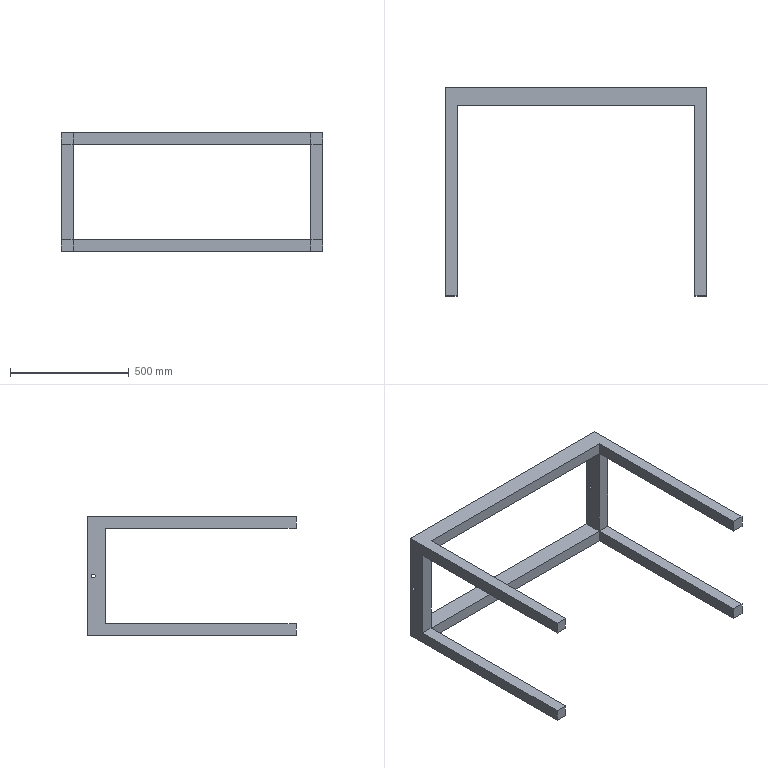Part | SolidWorks | features Cut 1, Extrusion 1, ICE 1 | 1 solid | 29 faces | box 1100 x 875 x 500 mm | volume 19232329 mm3 | plane 25 | cylinder 4 | commonest cylinder face diameters 15 x4
STEP:
#1=CARTESIAN_POINT('',(550.,52.5,-7.5));
#2=VERTEX_POINT('',#1);
#3=CARTESIAN_POINT('',(550.,52.5,7.5));
#4=VERTEX_POINT('',#3);
#5=CARTESIAN_POINT('',(550.,52.5,0.));
#6=DIRECTION('',(-1.,0.,0.));
#7=DIRECTION('',(0.,0.,1.));
#8=AXIS2_PLACEMENT_3D('',#5,#6,#7);
#9=CIRCLE('',#8,7.5);
#10=EDGE_CURVE('',#2,#4,#9,.T.);
#11=ORIENTED_EDGE('',*,*,#10,.F.);
#12=CARTESIAN_POINT('',(500.,52.5,-7.5));
#13=VERTEX_POINT('',#12);
#14=CARTESIAN_POINT('',(550.,52.5,-7.5));
#15=DIRECTION('',(-1.,0.,0.));
#16=VECTOR('',#15,1000.);
#17=LINE('',#14,#16);
#18=EDGE_CURVE('',#2,#13,#17,.T.);
#19=ORIENTED_EDGE('',*,*,#18,.T.);
#20=CARTESIAN_POINT('',(500.,52.5,7.5));
#21=VERTEX_POINT('',#20);
#22=CARTESIAN_POINT('',(500.,52.5,0.));
#23=DIRECTION('',(-1.,0.,0.));
#24=DIRECTION('',(0.,0.,1.));
#25=AXIS2_PLACEMENT_3D('',#22,#23,#24);
#26=CIRCLE('',#25,7.5);
#27=EDGE_CURVE('',#13,#21,#26,.T.);
#28=ORIENTED_EDGE('',*,*,#27,.T.);
#29=CARTESIAN_POINT('',(550.,52.5,7.5));
#30=DIRECTION('',(-1.,0.,0.));
#31=VECTOR('',#30,1000.);
#32=LINE('',#29,#31);
#33=EDGE_CURVE('',#4,#21,#32,.T.);
#34=ORIENTED_EDGE('',*,*,#33,.F.);
#35=EDGE_LOOP('',(#11,#19,#28,#34));
#36=FACE_OUTER_BOUND('',#35,.T.);
#37=CARTESIAN_POINT('',(550.,52.5,0.));
#38=DIRECTION('',(-1.,0.,0.));
#39=DIRECTION('',(0.,0.,1.));
#40=AXIS2_PLACEMENT_3D('',#37,#38,#39);
#41=CYLINDRICAL_SURFACE('',#40,7.5);
#42=ADVANCED_FACE('',(#36),#41,.F.);
#43=CARTESIAN_POINT('',(-500.,52.5,7.5));
#44=VERTEX_POINT('',#43);
#45=CARTESIAN_POINT('',(-500.,52.5,-7.5));
#46=VERTEX_POINT('',#45);
#47=CARTESIAN_POINT('',(-500.,52.5,0.));
#48=DIRECTION('',(1.,0.,0.));
#49=DIRECTION('',(0.,0.,-1.));
#50=AXIS2_PLACEMENT_3D('',#47,#48,#49);
#51=CIRCLE('',#50,7.5);
#52=EDGE_CURVE('',#44,#46,#51,.T.);
#53=ORIENTED_EDGE('',*,*,#52,.T.);
#54=CARTESIAN_POINT('',(-550.,52.5,-7.5));
#55=VERTEX_POINT('',#54);
#56=CARTESIAN_POINT('',(550.,52.5,-7.5));
#57=DIRECTION('',(-1.,0.,0.));
#58=VECTOR('',#57,1000.);
#59=LINE('',#56,#58);
#60=EDGE_CURVE('',#46,#55,#59,.T.);
#61=ORIENTED_EDGE('',*,*,#60,.T.);
#62=CARTESIAN_POINT('',(-550.,52.5,7.5));
#63=VERTEX_POINT('',#62);
#64=CARTESIAN_POINT('',(-550.,52.5,0.));
#65=DIRECTION('',(1.,0.,0.));
#66=DIRECTION('',(0.,0.,-1.));
#67=AXIS2_PLACEMENT_3D('',#64,#65,#66);
#68=CIRCLE('',#67,7.5);
#69=EDGE_CURVE('',#63,#55,#68,.T.);
#70=ORIENTED_EDGE('',*,*,#69,.F.);
#71=CARTESIAN_POINT('',(550.,52.5,7.5));
#72=DIRECTION('',(-1.,0.,0.));
#73=VECTOR('',#72,1000.);
#74=LINE('',#71,#73);
#75=EDGE_CURVE('',#44,#63,#74,.T.);
#76=ORIENTED_EDGE('',*,*,#75,.F.);
#77=EDGE_LOOP('',(#53,#61,#70,#76));
#78=FACE_OUTER_BOUND('',#77,.T.);
#79=CARTESIAN_POINT('',(550.,52.5,0.));
#80=DIRECTION('',(-1.,0.,0.));
#81=DIRECTION('',(0.,0.,1.));
#82=AXIS2_PLACEMENT_3D('',#79,#80,#81);
#83=CYLINDRICAL_SURFACE('',#82,7.5);
#84=ADVANCED_FACE('',(#78),#83,.F.);
#85=CARTESIAN_POINT('',(-500.,0.,-200.));
#86=VERTEX_POINT('',#85);
#87=CARTESIAN_POINT('',(-550.,0.,-200.));
#88=VERTEX_POINT('',#87);
#89=CARTESIAN_POINT('',(-550.,0.,-200.));
#90=DIRECTION('',(-1.,0.,0.));
#91=VECTOR('',#90,1000.);
#92=LINE('',#89,#91);
#93=EDGE_CURVE('',#86,#88,#92,.T.);
#94=ORIENTED_EDGE('',*,*,#93,.F.);
#95=CARTESIAN_POINT('',(-500.,0.,200.));
#96=VERTEX_POINT('',#95);
#97=CARTESIAN_POINT('',(-500.,0.,200.));
#98=DIRECTION('',(0.,0.,1.));
#99=VECTOR('',#98,1000.);
#100=LINE('',#97,#99);
#101=EDGE_CURVE('',#86,#96,#100,.T.);
#102=ORIENTED_EDGE('',*,*,#101,.T.);
#103=CARTESIAN_POINT('',(-550.,0.,200.));
#104=VERTEX_POINT('',#103);
#105=CARTESIAN_POINT('',(-550.,0.,200.));
#106=DIRECTION('',(1.,0.,0.));
#107=VECTOR('',#106,1000.);
#108=LINE('',#105,#107);
#109=EDGE_CURVE('',#104,#96,#108,.T.);
#110=ORIENTED_EDGE('',*,*,#109,.F.);
#111=CARTESIAN_POINT('',(-550.,0.,250.));
#112=DIRECTION('',(0.,0.,1.));
#113=VECTOR('',#112,1000.);
#114=LINE('',#111,#113);
#115=EDGE_CURVE('',#88,#104,#114,.T.);
#116=ORIENTED_EDGE('',*,*,#115,.F.);
#117=EDGE_LOOP('',(#94,#102,#110,#116));
#118=FACE_OUTER_BOUND('',#117,.T.);
#119=CARTESIAN_POINT('',(0.,0.,0.));
#120=DIRECTION('',(0.,-1.,0.));
#121=DIRECTION('',(0.,0.,-1.));
#122=AXIS2_PLACEMENT_3D('',#119,#120,#121);
#123=PLANE('',#122);
#124=ADVANCED_FACE('',(#118),#123,.T.);
#125=CARTESIAN_POINT('',(500.,0.,200.));
#126=VERTEX_POINT('',#125);
#127=CARTESIAN_POINT('',(550.,0.,200.));
#128=VERTEX_POINT('',#127);
#129=CARTESIAN_POINT('',(550.,0.,200.));
#130=DIRECTION('',(1.,0.,0.));
#131=VECTOR('',#130,1000.);
#132=LINE('',#129,#131);
#133=EDGE_CURVE('',#126,#128,#132,.T.);
#134=ORIENTED_EDGE('',*,*,#133,.F.);
#135=CARTESIAN_POINT('',(500.,0.,-200.));
#136=VERTEX_POINT('',#135);
#137=CARTESIAN_POINT('',(500.,0.,200.));
#138=DIRECTION('',(0.,0.,-1.));
#139=VECTOR('',#138,1000.);
#140=LINE('',#137,#139);
#141=EDGE_CURVE('',#126,#136,#140,.T.);
#142=ORIENTED_EDGE('',*,*,#141,.T.);
#143=CARTESIAN_POINT('',(550.,0.,-200.));
#144=VERTEX_POINT('',#143);
#145=CARTESIAN_POINT('',(550.,0.,-200.));
#146=DIRECTION('',(-1.,0.,0.));
#147=VECTOR('',#146,1000.);
#148=LINE('',#145,#147);
#149=EDGE_CURVE('',#144,#136,#148,.T.);
#150=ORIENTED_EDGE('',*,*,#149,.F.);
#151=CARTESIAN_POINT('',(550.,0.,250.));
#152=DIRECTION('',(0.,0.,-1.));
#153=VECTOR('',#152,1000.);
#154=LINE('',#151,#153);
#155=EDGE_CURVE('',#128,#144,#154,.T.);
#156=ORIENTED_EDGE('',*,*,#155,.F.);
#157=EDGE_LOOP('',(#134,#142,#150,#156));
#158=FACE_OUTER_BOUND('',#157,.T.);
#159=CARTESIAN_POINT('',(0.,0.,0.));
#160=DIRECTION('',(0.,-1.,0.));
#161=DIRECTION('',(0.,0.,-1.));
#162=AXIS2_PLACEMENT_3D('',#159,#160,#161);
#163=PLANE('',#162);
#164=ADVANCED_FACE('',(#158),#163,.T.);
#165=CARTESIAN_POINT('',(-500.,0.,-250.));
#166=VERTEX_POINT('',#165);
#167=CARTESIAN_POINT('',(-500.,0.,-250.));
#168=DIRECTION('',(0.,0.,1.));
#169=VECTOR('',#168,1000.);
#170=LINE('',#167,#169);
#171=EDGE_CURVE('',#166,#86,#170,.T.);
#172=ORIENTED_EDGE('',*,*,#171,.F.);
#173=CARTESIAN_POINT('',(500.,0.,-250.));
#174=VERTEX_POINT('',#173);
#175=CARTESIAN_POINT('',(-550.,0.,-250.));
#176=DIRECTION('',(-1.,0.,0.));
#177=VECTOR('',#176,1000.);
#178=LINE('',#175,#177);
#179=EDGE_CURVE('',#174,#166,#178,.T.);
#180=ORIENTED_EDGE('',*,*,#179,.F.);
#181=CARTESIAN_POINT('',(500.,0.,-250.));
#182=DIRECTION('',(0.,0.,-1.));
#183=VECTOR('',#182,1000.);
#184=LINE('',#181,#183);
#185=EDGE_CURVE('',#136,#174,#184,.T.);
#186=ORIENTED_EDGE('',*,*,#185,.F.);
#187=CARTESIAN_POINT('',(-500.,0.,-200.));
#188=DIRECTION('',(-1.,0.,0.));
#189=VECTOR('',#188,1000.);
#190=LINE('',#187,#189);
#191=EDGE_CURVE('',#136,#86,#190,.T.);
#192=ORIENTED_EDGE('',*,*,#191,.T.);
#193=EDGE_LOOP('',(#172,#180,#186,#192));
#194=FACE_OUTER_BOUND('',#193,.T.);
#195=CARTESIAN_POINT('',(0.,0.,0.));
#196=DIRECTION('',(0.,-1.,0.));
#197=DIRECTION('',(0.,0.,-1.));
#198=AXIS2_PLACEMENT_3D('',#195,#196,#197);
#199=PLANE('',#198);
#200=ADVANCED_FACE('',(#194),#199,.T.);
#201=CARTESIAN_POINT('',(550.,75.,250.));
#202=VERTEX_POINT('',#201);
#203=CARTESIAN_POINT('',(550.,75.,-250.));
#204=VERTEX_POINT('',#203);
#205=CARTESIAN_POINT('',(550.,75.,250.));
#206=DIRECTION('',(0.,0.,-1.));
#207=VECTOR('',#206,1000.);
#208=LINE('',#205,#207);
#209=EDGE_CURVE('',#202,#204,#208,.T.);
#210=ORIENTED_EDGE('',*,*,#209,.T.);
#211=CARTESIAN_POINT('',(-550.,75.,-250.));
#212=VERTEX_POINT('',#211);
#213=CARTESIAN_POINT('',(-550.,75.,-250.));
#214=DIRECTION('',(-1.,0.,0.));
#215=VECTOR('',#214,1000.);
#216=LINE('',#213,#215);
#217=EDGE_CURVE('',#204,#212,#216,.T.);
#218=ORIENTED_EDGE('',*,*,#217,.T.);
#219=CARTESIAN_POINT('',(-550.,75.,250.));
#220=VERTEX_POINT('',#219);
#221=CARTESIAN_POINT('',(-550.,75.,250.));
#222=DIRECTION('',(0.,0.,1.));
#223=VECTOR('',#222,1000.);
#224=LINE('',#221,#223);
#225=EDGE_CURVE('',#212,#220,#224,.T.);
#226=ORIENTED_EDGE('',*,*,#225,.T.);
#227=CARTESIAN_POINT('',(-550.,75.,250.));
#228=DIRECTION('',(1.,0.,0.));
#229=VECTOR('',#228,1000.);
#230=LINE('',#227,#229);
#231=EDGE_CURVE('',#220,#202,#230,.T.);
#232=ORIENTED_EDGE('',*,*,#231,.T.);
#233=EDGE_LOOP('',(#210,#218,#226,#232));
#234=FACE_OUTER_BOUND('',#233,.T.);
#235=CARTESIAN_POINT('',(500.,75.,200.));
#236=VERTEX_POINT('',#235);
#237=CARTESIAN_POINT('',(500.,75.,-200.));
#238=VERTEX_POINT('',#237);
#239=CARTESIAN_POINT('',(500.,75.,200.));
#240=DIRECTION('',(0.,0.,-1.));
#241=VECTOR('',#240,1000.);
#242=LINE('',#239,#241);
#243=EDGE_CURVE('',#236,#238,#242,.T.);
#244=ORIENTED_EDGE('',*,*,#243,.F.);
#245=CARTESIAN_POINT('',(-500.,75.,200.));
#246=VERTEX_POINT('',#245);
#247=CARTESIAN_POINT('',(-500.,75.,200.));
#248=DIRECTION('',(1.,0.,0.));
#249=VECTOR('',#248,1000.);
#250=LINE('',#247,#249);
#251=EDGE_CURVE('',#246,#236,#250,.T.);
#252=ORIENTED_EDGE('',*,*,#251,.F.);
#253=CARTESIAN_POINT('',(-500.,75.,-200.));
#254=VERTEX_POINT('',#253);
#255=CARTESIAN_POINT('',(-500.,75.,200.));
#256=DIRECTION('',(0.,0.,1.));
#257=VECTOR('',#256,1000.);
#258=LINE('',#255,#257);
#259=EDGE_CURVE('',#254,#246,#258,.T.);
#260=ORIENTED_EDGE('',*,*,#259,.F.);
#261=CARTESIAN_POINT('',(-500.,75.,-200.));
#262=DIRECTION('',(-1.,0.,0.));
#263=VECTOR('',#262,1000.);
#264=LINE('',#261,#263);
#265=EDGE_CURVE('',#238,#254,#264,.T.);
#266=ORIENTED_EDGE('',*,*,#265,.F.);
#267=EDGE_LOOP('',(#244,#252,#260,#266));
#268=FACE_BOUND('',#267,.T.);
#269=CARTESIAN_POINT('',(0.,75.,0.));
#270=DIRECTION('',(0.,-1.,0.));
#271=DIRECTION('',(0.,0.,-1.));
#272=AXIS2_PLACEMENT_3D('',#269,#270,#271);
#273=PLANE('',#272);
#274=ADVANCED_FACE('',(#234,#268),#273,.F.);
#275=CARTESIAN_POINT('',(500.,0.,250.));
#276=VERTEX_POINT('',#275);
#277=CARTESIAN_POINT('',(500.,0.,250.));
#278=DIRECTION('',(0.,0.,-1.));
#279=VECTOR('',#278,1000.);
#280=LINE('',#277,#279);
#281=EDGE_CURVE('',#276,#126,#280,.T.);
#282=ORIENTED_EDGE('',*,*,#281,.F.);
#283=CARTESIAN_POINT('',(-500.,0.,250.));
#284=VERTEX_POINT('',#283);
#285=CARTESIAN_POINT('',(-550.,0.,250.));
#286=DIRECTION('',(1.,0.,0.));
#287=VECTOR('',#286,1000.);
#288=LINE('',#285,#287);
#289=EDGE_CURVE('',#284,#276,#288,.T.);
#290=ORIENTED_EDGE('',*,*,#289,.F.);
#291=CARTESIAN_POINT('',(-500.,0.,250.));
#292=DIRECTION('',(0.,0.,1.));
#293=VECTOR('',#292,1000.);
#294=LINE('',#291,#293);
#295=EDGE_CURVE('',#96,#284,#294,.T.);
#296=ORIENTED_EDGE('',*,*,#295,.F.);
#297=CARTESIAN_POINT('',(-500.,0.,200.));
#298=DIRECTION('',(1.,0.,0.));
#299=VECTOR('',#298,1000.);
#300=LINE('',#297,#299);
#301=EDGE_CURVE('',#96,#126,#300,.T.);
#302=ORIENTED_EDGE('',*,*,#301,.T.);
#303=EDGE_LOOP('',(#282,#290,#296,#302));
#304=FACE_OUTER_BOUND('',#303,.T.);
#305=CARTESIAN_POINT('',(0.,0.,0.));
#306=DIRECTION('',(0.,-1.,0.));
#307=DIRECTION('',(0.,0.,-1.));
#308=AXIS2_PLACEMENT_3D('',#305,#306,#307);
#309=PLANE('',#308);
#310=ADVANCED_FACE('',(#304),#309,.T.);
#311=CARTESIAN_POINT('',(550.,52.5,0.));
#312=DIRECTION('',(-1.,0.,0.));
#313=DIRECTION('',(0.,0.,1.));
#314=AXIS2_PLACEMENT_3D('',#311,#312,#313);
#315=CIRCLE('',#314,7.5);
#316=EDGE_CURVE('',#4,#2,#315,.T.);
#317=ORIENTED_EDGE('',*,*,#316,.T.);
#318=ORIENTED_EDGE('',*,*,#10,.T.);
#319=EDGE_LOOP('',(#317,#318));
#320=FACE_BOUND('',#319,.T.);
#321=CARTESIAN_POINT('',(550.,-800.,250.));
#322=VERTEX_POINT('',#321);
#323=CARTESIAN_POINT('',(550.,75.,250.));
#324=DIRECTION('',(0.,-1.,0.));
#325=VECTOR('',#324,1000.);
#326=LINE('',#323,#325);
#327=EDGE_CURVE('',#202,#322,#326,.T.);
#328=ORIENTED_EDGE('',*,*,#327,.T.);
#329=CARTESIAN_POINT('',(550.,-800.,200.));
#330=VERTEX_POINT('',#329);
#331=CARTESIAN_POINT('',(550.,-800.,250.));
#332=DIRECTION('',(0.,0.,1.));
#333=VECTOR('',#332,1000.);
#334=LINE('',#331,#333);
#335=EDGE_CURVE('',#330,#322,#334,.T.);
#336=ORIENTED_EDGE('',*,*,#335,.F.);
#337=CARTESIAN_POINT('',(550.,-800.,200.));
#338=DIRECTION('',(0.,1.,0.));
#339=VECTOR('',#338,1000.);
#340=LINE('',#337,#339);
#341=EDGE_CURVE('',#330,#128,#340,.T.);
#342=ORIENTED_EDGE('',*,*,#341,.T.);
#343=ORIENTED_EDGE('',*,*,#155,.T.);
#344=CARTESIAN_POINT('',(550.,-800.,-200.));
#345=VERTEX_POINT('',#344);
#346=CARTESIAN_POINT('',(550.,-800.,-200.));
#347=DIRECTION('',(0.,1.,0.));
#348=VECTOR('',#347,1000.);
#349=LINE('',#346,#348);
#350=EDGE_CURVE('',#345,#144,#349,.T.);
#351=ORIENTED_EDGE('',*,*,#350,.F.);
#352=CARTESIAN_POINT('',(550.,-800.,-250.));
#353=VERTEX_POINT('',#352);
#354=CARTESIAN_POINT('',(550.,-800.,-250.));
#355=DIRECTION('',(0.,0.,1.));
#356=VECTOR('',#355,1000.);
#357=LINE('',#354,#356);
#358=EDGE_CURVE('',#353,#345,#357,.T.);
#359=ORIENTED_EDGE('',*,*,#358,.F.);
#360=CARTESIAN_POINT('',(550.,75.,-250.));
#361=DIRECTION('',(0.,-1.,0.));
#362=VECTOR('',#361,1000.);
#363=LINE('',#360,#362);
#364=EDGE_CURVE('',#204,#353,#363,.T.);
#365=ORIENTED_EDGE('',*,*,#364,.F.);
#366=ORIENTED_EDGE('',*,*,#209,.F.);
#367=EDGE_LOOP('',(#328,#336,#342,#343,#351,#359,#365,#366));
#368=FACE_OUTER_BOUND('',#367,.T.);
#369=CARTESIAN_POINT('',(550.,75.,250.));
#370=DIRECTION('',(-1.,0.,0.));
#371=DIRECTION('',(0.,0.,1.));
#372=AXIS2_PLACEMENT_3D('',#369,#370,#371);
#373=PLANE('',#372);
#374=ADVANCED_FACE('',(#320,#368),#373,.F.);
#375=ORIENTED_EDGE('',*,*,#364,.T.);
#376=CARTESIAN_POINT('',(500.,-800.,-250.));
#377=VERTEX_POINT('',#376);
#378=CARTESIAN_POINT('',(550.,-800.,-250.));
#379=DIRECTION('',(1.,0.,0.));
#380=VECTOR('',#379,1000.);
#381=LINE('',#378,#380);
#382=EDGE_CURVE('',#377,#353,#381,.T.);
#383=ORIENTED_EDGE('',*,*,#382,.F.);
#384=CARTESIAN_POINT('',(500.,-800.,-250.));
#385=DIRECTION('',(0.,1.,0.));
#386=VECTOR('',#385,1000.);
#387=LINE('',#384,#386);
#388=EDGE_CURVE('',#377,#174,#387,.T.);
#389=ORIENTED_EDGE('',*,*,#388,.T.);
#390=ORIENTED_EDGE('',*,*,#179,.T.);
#391=CARTESIAN_POINT('',(-500.,-800.,-250.));
#392=VERTEX_POINT('',#391);
#393=CARTESIAN_POINT('',(-500.,-800.,-250.));
#394=DIRECTION('',(0.,1.,0.));
#395=VECTOR('',#394,1000.);
#396=LINE('',#393,#395);
#397=EDGE_CURVE('',#392,#166,#396,.T.);
#398=ORIENTED_EDGE('',*,*,#397,.F.);
#399=CARTESIAN_POINT('',(-550.,-800.,-250.));
#400=VERTEX_POINT('',#399);
#401=CARTESIAN_POINT('',(-550.,-800.,-250.));
#402=DIRECTION('',(1.,0.,0.));
#403=VECTOR('',#402,1000.);
#404=LINE('',#401,#403);
#405=EDGE_CURVE('',#400,#392,#404,.T.);
#406=ORIENTED_EDGE('',*,*,#405,.F.);
#407=CARTESIAN_POINT('',(-550.,75.,-250.));
#408=DIRECTION('',(0.,-1.,0.));
#409=VECTOR('',#408,1000.);
#410=LINE('',#407,#409);
#411=EDGE_CURVE('',#212,#400,#410,.T.);
#412=ORIENTED_EDGE('',*,*,#411,.F.);
#413=ORIENTED_EDGE('',*,*,#217,.F.);
#414=EDGE_LOOP('',(#375,#383,#389,#390,#398,#406,#412,#413));
#415=FACE_OUTER_BOUND('',#414,.T.);
#416=CARTESIAN_POINT('',(-550.,75.,-250.));
#417=DIRECTION('',(0.,0.,1.));
#418=DIRECTION('',(1.,0.,0.));
#419=AXIS2_PLACEMENT_3D('',#416,#417,#418);
#420=PLANE('',#419);
#421=ADVANCED_FACE('',(#415),#420,.F.);
#422=ORIENTED_EDGE('',*,*,#69,.T.);
#423=CARTESIAN_POINT('',(-550.,52.5,0.));
#424=DIRECTION('',(1.,0.,0.));
#425=DIRECTION('',(0.,0.,-1.));
#426=AXIS2_PLACEMENT_3D('',#423,#424,#425);
#427=CIRCLE('',#426,7.5);
#428=EDGE_CURVE('',#55,#63,#427,.T.);
#429=ORIENTED_EDGE('',*,*,#428,.T.);
#430=EDGE_LOOP('',(#422,#429));
#431=FACE_BOUND('',#430,.T.);
#432=ORIENTED_EDGE('',*,*,#411,.T.);
#433=CARTESIAN_POINT('',(-550.,-800.,-200.));
#434=VERTEX_POINT('',#433);
#435=CARTESIAN_POINT('',(-550.,-800.,-250.));
#436=DIRECTION('',(0.,0.,-1.));
#437=VECTOR('',#436,1000.);
#438=LINE('',#435,#437);
#439=EDGE_CURVE('',#434,#400,#438,.T.);
#440=ORIENTED_EDGE('',*,*,#439,.F.);
#441=CARTESIAN_POINT('',(-550.,-800.,-200.));
#442=DIRECTION('',(0.,1.,0.));
#443=VECTOR('',#442,1000.);
#444=LINE('',#441,#443);
#445=EDGE_CURVE('',#434,#88,#444,.T.);
#446=ORIENTED_EDGE('',*,*,#445,.T.);
#447=ORIENTED_EDGE('',*,*,#115,.T.);
#448=CARTESIAN_POINT('',(-550.,-800.,200.));
#449=VERTEX_POINT('',#448);
#450=CARTESIAN_POINT('',(-550.,-800.,200.));
#451=DIRECTION('',(0.,1.,0.));
#452=VECTOR('',#451,1000.);
#453=LINE('',#450,#452);
#454=EDGE_CURVE('',#449,#104,#453,.T.);
#455=ORIENTED_EDGE('',*,*,#454,.F.);
#456=CARTESIAN_POINT('',(-550.,-800.,250.));
#457=VERTEX_POINT('',#456);
#458=CARTESIAN_POINT('',(-550.,-800.,250.));
#459=DIRECTION('',(0.,0.,-1.));
#460=VECTOR('',#459,1000.);
#461=LINE('',#458,#460);
#462=EDGE_CURVE('',#457,#449,#461,.T.);
#463=ORIENTED_EDGE('',*,*,#462,.F.);
#464=CARTESIAN_POINT('',(-550.,75.,250.));
#465=DIRECTION('',(0.,-1.,0.));
#466=VECTOR('',#465,1000.);
#467=LINE('',#464,#466);
#468=EDGE_CURVE('',#220,#457,#467,.T.);
#469=ORIENTED_EDGE('',*,*,#468,.F.);
#470=ORIENTED_EDGE('',*,*,#225,.F.);
#471=EDGE_LOOP('',(#432,#440,#446,#447,#455,#463,#469,#470));
#472=FACE_OUTER_BOUND('',#471,.T.);
#473=CARTESIAN_POINT('',(-550.,75.,250.));
#474=DIRECTION('',(1.,0.,0.));
#475=DIRECTION('',(0.,0.,-1.));
#476=AXIS2_PLACEMENT_3D('',#473,#474,#475);
#477=PLANE('',#476);
#478=ADVANCED_FACE('',(#431,#472),#477,.F.);
#479=ORIENTED_EDGE('',*,*,#468,.T.);
#480=CARTESIAN_POINT('',(-500.,-800.,250.));
#481=VERTEX_POINT('',#480);
#482=CARTESIAN_POINT('',(-550.,-800.,250.));
#483=DIRECTION('',(-1.,0.,0.));
#484=VECTOR('',#483,1000.);
#485=LINE('',#482,#484);
#486=EDGE_CURVE('',#481,#457,#485,.T.);
#487=ORIENTED_EDGE('',*,*,#486,.F.);
#488=CARTESIAN_POINT('',(-500.,-800.,250.));
#489=DIRECTION('',(0.,1.,0.));
#490=VECTOR('',#489,1000.);
#491=LINE('',#488,#490);
#492=EDGE_CURVE('',#481,#284,#491,.T.);
#493=ORIENTED_EDGE('',*,*,#492,.T.);
#494=ORIENTED_EDGE('',*,*,#289,.T.);
#495=CARTESIAN_POINT('',(500.,-800.,250.));
#496=VERTEX_POINT('',#495);
#497=CARTESIAN_POINT('',(500.,-800.,250.));
#498=DIRECTION('',(0.,1.,0.));
#499=VECTOR('',#498,1000.);
#500=LINE('',#497,#499);
#501=EDGE_CURVE('',#496,#276,#500,.T.);
#502=ORIENTED_EDGE('',*,*,#501,.F.);
#503=CARTESIAN_POINT('',(550.,-800.,250.));
#504=DIRECTION('',(-1.,0.,0.));
#505=VECTOR('',#504,1000.);
#506=LINE('',#503,#505);
#507=EDGE_CURVE('',#322,#496,#506,.T.);
#508=ORIENTED_EDGE('',*,*,#507,.F.);
#509=ORIENTED_EDGE('',*,*,#327,.F.);
#510=ORIENTED_EDGE('',*,*,#231,.F.);
#511=EDGE_LOOP('',(#479,#487,#493,#494,#502,#508,#509,#510));
#512=FACE_OUTER_BOUND('',#511,.T.);
#513=CARTESIAN_POINT('',(-550.,75.,250.));
#514=DIRECTION('',(0.,0.,-1.));
#515=DIRECTION('',(-1.,0.,0.));
#516=AXIS2_PLACEMENT_3D('',#513,#514,#515);
#517=PLANE('',#516);
#518=ADVANCED_FACE('',(#512),#517,.F.);
#519=CARTESIAN_POINT('',(500.,52.5,0.));
#520=DIRECTION('',(-1.,0.,0.));
#521=DIRECTION('',(0.,0.,1.));
#522=AXIS2_PLACEMENT_3D('',#519,#520,#521);
#523=CIRCLE('',#522,7.5);
#524=EDGE_CURVE('',#21,#13,#523,.T.);
#525=ORIENTED_EDGE('',*,*,#524,.F.);
#526=ORIENTED_EDGE('',*,*,#27,.F.);
#527=EDGE_LOOP('',(#525,#526));
#528=FACE_BOUND('',#527,.T.);
#529=ORIENTED_EDGE('',*,*,#141,.F.);
#530=CARTESIAN_POINT('',(500.,75.,200.));
#531=DIRECTION('',(0.,-1.,0.));
#532=VECTOR('',#531,1000.);
#533=LINE('',#530,#532);
#534=EDGE_CURVE('',#236,#126,#533,.T.);
#535=ORIENTED_EDGE('',*,*,#534,.F.);
#536=ORIENTED_EDGE('',*,*,#243,.T.);
#537=CARTESIAN_POINT('',(500.,75.,-200.));
#538=DIRECTION('',(0.,-1.,0.));
#539=VECTOR('',#538,1000.);
#540=LINE('',#537,#539);
#541=EDGE_CURVE('',#238,#136,#540,.T.);
#542=ORIENTED_EDGE('',*,*,#541,.T.);
#543=EDGE_LOOP('',(#529,#535,#536,#542));
#544=FACE_OUTER_BOUND('',#543,.T.);
#545=CARTESIAN_POINT('',(500.,75.,200.));
#546=DIRECTION('',(-1.,0.,0.));
#547=DIRECTION('',(0.,0.,1.));
#548=AXIS2_PLACEMENT_3D('',#545,#546,#547);
#549=PLANE('',#548);
#550=ADVANCED_FACE('',(#528,#544),#549,.T.);
#551=ORIENTED_EDGE('',*,*,#191,.F.);
#552=ORIENTED_EDGE('',*,*,#541,.F.);
#553=ORIENTED_EDGE('',*,*,#265,.T.);
#554=CARTESIAN_POINT('',(-500.,75.,-200.));
#555=DIRECTION('',(0.,-1.,0.));
#556=VECTOR('',#555,1000.);
#557=LINE('',#554,#556);
#558=EDGE_CURVE('',#254,#86,#557,.T.);
#559=ORIENTED_EDGE('',*,*,#558,.T.);
#560=EDGE_LOOP('',(#551,#552,#553,#559));
#561=FACE_OUTER_BOUND('',#560,.T.);
#562=CARTESIAN_POINT('',(-500.,75.,-200.));
#563=DIRECTION('',(0.,0.,1.));
#564=DIRECTION('',(1.,0.,0.));
#565=AXIS2_PLACEMENT_3D('',#562,#563,#564);
#566=PLANE('',#565);
#567=ADVANCED_FACE('',(#561),#566,.T.);
#568=ORIENTED_EDGE('',*,*,#52,.F.);
#569=CARTESIAN_POINT('',(-500.,52.5,0.));
#570=DIRECTION('',(1.,0.,0.));
#571=DIRECTION('',(0.,0.,-1.));
#572=AXIS2_PLACEMENT_3D('',#569,#570,#571);
#573=CIRCLE('',#572,7.5);
#574=EDGE_CURVE('',#46,#44,#573,.T.);
#575=ORIENTED_EDGE('',*,*,#574,.F.);
#576=EDGE_LOOP('',(#568,#575));
#577=FACE_BOUND('',#576,.T.);
#578=ORIENTED_EDGE('',*,*,#101,.F.);
#579=ORIENTED_EDGE('',*,*,#558,.F.);
#580=ORIENTED_EDGE('',*,*,#259,.T.);
#581=CARTESIAN_POINT('',(-500.,75.,200.));
#582=DIRECTION('',(0.,-1.,0.));
#583=VECTOR('',#582,1000.);
#584=LINE('',#581,#583);
#585=EDGE_CURVE('',#246,#96,#584,.T.);
#586=ORIENTED_EDGE('',*,*,#585,.T.);
#587=EDGE_LOOP('',(#578,#579,#580,#586));
#588=FACE_OUTER_BOUND('',#587,.T.);
#589=CARTESIAN_POINT('',(-500.,75.,200.));
#590=DIRECTION('',(1.,0.,0.));
#591=DIRECTION('',(0.,0.,-1.));
#592=AXIS2_PLACEMENT_3D('',#589,#590,#591);
#593=PLANE('',#592);
#594=ADVANCED_FACE('',(#577,#588),#593,.T.);
#595=ORIENTED_EDGE('',*,*,#301,.F.);
#596=ORIENTED_EDGE('',*,*,#585,.F.);
#597=ORIENTED_EDGE('',*,*,#251,.T.);
#598=ORIENTED_EDGE('',*,*,#534,.T.);
#599=EDGE_LOOP('',(#595,#596,#597,#598));
#600=FACE_OUTER_BOUND('',#599,.T.);
#601=CARTESIAN_POINT('',(-500.,75.,200.));
#602=DIRECTION('',(0.,0.,-1.));
#603=DIRECTION('',(-1.,0.,0.));
#604=AXIS2_PLACEMENT_3D('',#601,#602,#603);
#605=PLANE('',#604);
#606=ADVANCED_FACE('',(#600),#605,.T.);
#607=ORIENTED_EDGE('',*,*,#109,.T.);
#608=CARTESIAN_POINT('',(-500.,-800.,200.));
#609=VERTEX_POINT('',#608);
#610=CARTESIAN_POINT('',(-500.,-800.,200.));
#611=DIRECTION('',(0.,1.,0.));
#612=VECTOR('',#611,1000.);
#613=LINE('',#610,#612);
#614=EDGE_CURVE('',#609,#96,#613,.T.);
#615=ORIENTED_EDGE('',*,*,#614,.F.);
#616=CARTESIAN_POINT('',(-550.,-800.,200.));
#617=DIRECTION('',(1.,0.,0.));
#618=VECTOR('',#617,1000.);
#619=LINE('',#616,#618);
#620=EDGE_CURVE('',#449,#609,#619,.T.);
#621=ORIENTED_EDGE('',*,*,#620,.F.);
#622=ORIENTED_EDGE('',*,*,#454,.T.);
#623=EDGE_LOOP('',(#607,#615,#621,#622));
#624=FACE_OUTER_BOUND('',#623,.T.);
#625=CARTESIAN_POINT('',(-550.,-800.,200.));
#626=DIRECTION('',(0.,0.,1.));
#627=DIRECTION('',(1.,0.,0.));
#628=AXIS2_PLACEMENT_3D('',#625,#626,#627);
#629=PLANE('',#628);
#630=ADVANCED_FACE('',(#624),#629,.F.);
#631=ORIENTED_EDGE('',*,*,#295,.T.);
#632=ORIENTED_EDGE('',*,*,#492,.F.);
#633=CARTESIAN_POINT('',(-500.,-800.,250.));
#634=DIRECTION('',(0.,0.,1.));
#635=VECTOR('',#634,1000.);
#636=LINE('',#633,#635);
#637=EDGE_CURVE('',#609,#481,#636,.T.);
#638=ORIENTED_EDGE('',*,*,#637,.F.);
#639=ORIENTED_EDGE('',*,*,#614,.T.);
#640=EDGE_LOOP('',(#631,#632,#638,#639));
#641=FACE_OUTER_BOUND('',#640,.T.);
#642=CARTESIAN_POINT('',(-500.,-800.,250.));
#643=DIRECTION('',(-1.,0.,0.));
#644=DIRECTION('',(0.,0.,1.));
#645=AXIS2_PLACEMENT_3D('',#642,#643,#644);
#646=PLANE('',#645);
#647=ADVANCED_FACE('',(#641),#646,.F.);
#648=ORIENTED_EDGE('',*,*,#462,.T.);
#649=ORIENTED_EDGE('',*,*,#620,.T.);
#650=ORIENTED_EDGE('',*,*,#637,.T.);
#651=ORIENTED_EDGE('',*,*,#486,.T.);
#652=EDGE_LOOP('',(#648,#649,#650,#651));
#653=FACE_OUTER_BOUND('',#652,.T.);
#654=CARTESIAN_POINT('',(0.,-800.,0.));
#655=DIRECTION('',(0.,-1.,0.));
#656=DIRECTION('',(0.,0.,-1.));
#657=AXIS2_PLACEMENT_3D('',#654,#655,#656);
#658=PLANE('',#657);
#659=ADVANCED_FACE('',(#653),#658,.T.);
#660=ORIENTED_EDGE('',*,*,#149,.T.);
#661=CARTESIAN_POINT('',(500.,-800.,-200.));
#662=VERTEX_POINT('',#661);
#663=CARTESIAN_POINT('',(500.,-800.,-200.));
#664=DIRECTION('',(0.,1.,0.));
#665=VECTOR('',#664,1000.);
#666=LINE('',#663,#665);
#667=EDGE_CURVE('',#662,#136,#666,.T.);
#668=ORIENTED_EDGE('',*,*,#667,.F.);
#669=CARTESIAN_POINT('',(550.,-800.,-200.));
#670=DIRECTION('',(-1.,0.,0.));
#671=VECTOR('',#670,1000.);
#672=LINE('',#669,#671);
#673=EDGE_CURVE('',#345,#662,#672,.T.);
#674=ORIENTED_EDGE('',*,*,#673,.F.);
#675=ORIENTED_EDGE('',*,*,#350,.T.);
#676=EDGE_LOOP('',(#660,#668,#674,#675));
#677=FACE_OUTER_BOUND('',#676,.T.);
#678=CARTESIAN_POINT('',(550.,-800.,-200.));
#679=DIRECTION('',(0.,0.,-1.));
#680=DIRECTION('',(-1.,0.,0.));
#681=AXIS2_PLACEMENT_3D('',#678,#679,#680);
#682=PLANE('',#681);
#683=ADVANCED_FACE('',(#677),#682,.F.);
#684=ORIENTED_EDGE('',*,*,#185,.T.);
#685=ORIENTED_EDGE('',*,*,#388,.F.);
#686=CARTESIAN_POINT('',(500.,-800.,-250.));
#687=DIRECTION('',(0.,0.,-1.));
#688=VECTOR('',#687,1000.);
#689=LINE('',#686,#688);
#690=EDGE_CURVE('',#662,#377,#689,.T.);
#691=ORIENTED_EDGE('',*,*,#690,.F.);
#692=ORIENTED_EDGE('',*,*,#667,.T.);
#693=EDGE_LOOP('',(#684,#685,#691,#692));
#694=FACE_OUTER_BOUND('',#693,.T.);
#695=CARTESIAN_POINT('',(500.,-800.,-250.));
#696=DIRECTION('',(1.,0.,0.));
#697=DIRECTION('',(0.,0.,-1.));
#698=AXIS2_PLACEMENT_3D('',#695,#696,#697);
#699=PLANE('',#698);
#700=ADVANCED_FACE('',(#694),#699,.F.);
#701=ORIENTED_EDGE('',*,*,#358,.T.);
#702=ORIENTED_EDGE('',*,*,#673,.T.);
#703=ORIENTED_EDGE('',*,*,#690,.T.);
#704=ORIENTED_EDGE('',*,*,#382,.T.);
#705=EDGE_LOOP('',(#701,#702,#703,#704));
#706=FACE_OUTER_BOUND('',#705,.T.);
#707=CARTESIAN_POINT('',(0.,-800.,0.));
#708=DIRECTION('',(0.,-1.,0.));
#709=DIRECTION('',(0.,0.,-1.));
#710=AXIS2_PLACEMENT_3D('',#707,#708,#709);
#711=PLANE('',#710);
#712=ADVANCED_FACE('',(#706),#711,.T.);
#713=ORIENTED_EDGE('',*,*,#281,.T.);
#714=CARTESIAN_POINT('',(500.,-800.,200.));
#715=VERTEX_POINT('',#714);
#716=CARTESIAN_POINT('',(500.,-800.,200.));
#717=DIRECTION('',(0.,1.,0.));
#718=VECTOR('',#717,1000.);
#719=LINE('',#716,#718);
#720=EDGE_CURVE('',#715,#126,#719,.T.);
#721=ORIENTED_EDGE('',*,*,#720,.F.);
#722=CARTESIAN_POINT('',(500.,-800.,250.));
#723=DIRECTION('',(0.,0.,-1.));
#724=VECTOR('',#723,1000.);
#725=LINE('',#722,#724);
#726=EDGE_CURVE('',#496,#715,#725,.T.);
#727=ORIENTED_EDGE('',*,*,#726,.F.);
#728=ORIENTED_EDGE('',*,*,#501,.T.);
#729=EDGE_LOOP('',(#713,#721,#727,#728));
#730=FACE_OUTER_BOUND('',#729,.T.);
#731=CARTESIAN_POINT('',(500.,-800.,250.));
#732=DIRECTION('',(1.,0.,0.));
#733=DIRECTION('',(0.,0.,-1.));
#734=AXIS2_PLACEMENT_3D('',#731,#732,#733);
#735=PLANE('',#734);
#736=ADVANCED_FACE('',(#730),#735,.F.);
#737=ORIENTED_EDGE('',*,*,#133,.T.);
#738=ORIENTED_EDGE('',*,*,#341,.F.);
#739=CARTESIAN_POINT('',(550.,-800.,200.));
#740=DIRECTION('',(1.,0.,0.));
#741=VECTOR('',#740,1000.);
#742=LINE('',#739,#741);
#743=EDGE_CURVE('',#715,#330,#742,.T.);
#744=ORIENTED_EDGE('',*,*,#743,.F.);
#745=ORIENTED_EDGE('',*,*,#720,.T.);
#746=EDGE_LOOP('',(#737,#738,#744,#745));
#747=FACE_OUTER_BOUND('',#746,.T.);
#748=CARTESIAN_POINT('',(550.,-800.,200.));
#749=DIRECTION('',(0.,0.,1.));
#750=DIRECTION('',(1.,0.,0.));
#751=AXIS2_PLACEMENT_3D('',#748,#749,#750);
#752=PLANE('',#751);
#753=ADVANCED_FACE('',(#747),#752,.F.);
#754=ORIENTED_EDGE('',*,*,#507,.T.);
#755=ORIENTED_EDGE('',*,*,#726,.T.);
#756=ORIENTED_EDGE('',*,*,#743,.T.);
#757=ORIENTED_EDGE('',*,*,#335,.T.);
#758=EDGE_LOOP('',(#754,#755,#756,#757));
#759=FACE_OUTER_BOUND('',#758,.T.);
#760=CARTESIAN_POINT('',(0.,-800.,0.));
#761=DIRECTION('',(0.,-1.,0.));
#762=DIRECTION('',(0.,0.,-1.));
#763=AXIS2_PLACEMENT_3D('',#760,#761,#762);
#764=PLANE('',#763);
#765=ADVANCED_FACE('',(#759),#764,.T.);
#766=ORIENTED_EDGE('',*,*,#171,.T.);
#767=CARTESIAN_POINT('',(-500.,-800.,-200.));
#768=VERTEX_POINT('',#767);
#769=CARTESIAN_POINT('',(-500.,-800.,-200.));
#770=DIRECTION('',(0.,1.,0.));
#771=VECTOR('',#770,1000.);
#772=LINE('',#769,#771);
#773=EDGE_CURVE('',#768,#86,#772,.T.);
#774=ORIENTED_EDGE('',*,*,#773,.F.);
#775=CARTESIAN_POINT('',(-500.,-800.,-250.));
#776=DIRECTION('',(0.,0.,1.));
#777=VECTOR('',#776,1000.);
#778=LINE('',#775,#777);
#779=EDGE_CURVE('',#392,#768,#778,.T.);
#780=ORIENTED_EDGE('',*,*,#779,.F.);
#781=ORIENTED_EDGE('',*,*,#397,.T.);
#782=EDGE_LOOP('',(#766,#774,#780,#781));
#783=FACE_OUTER_BOUND('',#782,.T.);
#784=CARTESIAN_POINT('',(-500.,-800.,-250.));
#785=DIRECTION('',(-1.,0.,0.));
#786=DIRECTION('',(0.,0.,1.));
#787=AXIS2_PLACEMENT_3D('',#784,#785,#786);
#788=PLANE('',#787);
#789=ADVANCED_FACE('',(#783),#788,.F.);
#790=ORIENTED_EDGE('',*,*,#93,.T.);
#791=ORIENTED_EDGE('',*,*,#445,.F.);
#792=CARTESIAN_POINT('',(-550.,-800.,-200.));
#793=DIRECTION('',(-1.,0.,0.));
#794=VECTOR('',#793,1000.);
#795=LINE('',#792,#794);
#796=EDGE_CURVE('',#768,#434,#795,.T.);
#797=ORIENTED_EDGE('',*,*,#796,.F.);
#798=ORIENTED_EDGE('',*,*,#773,.T.);
#799=EDGE_LOOP('',(#790,#791,#797,#798));
#800=FACE_OUTER_BOUND('',#799,.T.);
#801=CARTESIAN_POINT('',(-550.,-800.,-200.));
#802=DIRECTION('',(0.,0.,-1.));
#803=DIRECTION('',(-1.,0.,0.));
#804=AXIS2_PLACEMENT_3D('',#801,#802,#803);
#805=PLANE('',#804);
#806=ADVANCED_FACE('',(#800),#805,.F.);
#807=ORIENTED_EDGE('',*,*,#405,.T.);
#808=ORIENTED_EDGE('',*,*,#779,.T.);
#809=ORIENTED_EDGE('',*,*,#796,.T.);
#810=ORIENTED_EDGE('',*,*,#439,.T.);
#811=EDGE_LOOP('',(#807,#808,#809,#810));
#812=FACE_OUTER_BOUND('',#811,.T.);
#813=CARTESIAN_POINT('',(0.,-800.,0.));
#814=DIRECTION('',(0.,-1.,0.));
#815=DIRECTION('',(0.,0.,-1.));
#816=AXIS2_PLACEMENT_3D('',#813,#814,#815);
#817=PLANE('',#816);
#818=ADVANCED_FACE('',(#812),#817,.T.);
#819=ORIENTED_EDGE('',*,*,#60,.F.);
#820=ORIENTED_EDGE('',*,*,#574,.T.);
#821=ORIENTED_EDGE('',*,*,#75,.T.);
#822=ORIENTED_EDGE('',*,*,#428,.F.);
#823=EDGE_LOOP('',(#819,#820,#821,#822));
#824=FACE_OUTER_BOUND('',#823,.T.);
#825=CARTESIAN_POINT('',(550.,52.5,0.));
#826=DIRECTION('',(-1.,0.,0.));
#827=DIRECTION('',(0.,0.,1.));
#828=AXIS2_PLACEMENT_3D('',#825,#826,#827);
#829=CYLINDRICAL_SURFACE('',#828,7.5);
#830=ADVANCED_FACE('',(#824),#829,.F.);
#831=ORIENTED_EDGE('',*,*,#18,.F.);
#832=ORIENTED_EDGE('',*,*,#316,.F.);
#833=ORIENTED_EDGE('',*,*,#33,.T.);
#834=ORIENTED_EDGE('',*,*,#524,.T.);
#835=EDGE_LOOP('',(#831,#832,#833,#834));
#836=FACE_OUTER_BOUND('',#835,.T.);
#837=CARTESIAN_POINT('',(550.,52.5,0.));
#838=DIRECTION('',(-1.,0.,0.));
#839=DIRECTION('',(0.,0.,1.));
#840=AXIS2_PLACEMENT_3D('',#837,#838,#839);
#841=CYLINDRICAL_SURFACE('',#840,7.5);
#842=ADVANCED_FACE('',(#836),#841,.F.);
#843=CLOSED_SHELL('',(#42,#84,#124,#164,#200,#274,#310,#374,#421,#478,#518,#550,#567,#594,#606,#630,#647,#659,#683,#700,#712,#736,#753,#765,#789,#806,#818,#830,#842));
#844=MANIFOLD_SOLID_BREP('',#843);
#845=CARTESIAN_POINT('',(0.,0.,0.));
#846=DIRECTION('',(0.,0.,1.));
#847=DIRECTION('',(1.,0.,0.));
#848=AXIS2_PLACEMENT_3D('',#845,#846,#847);
#849=(LENGTH_UNIT()NAMED_UNIT(*)SI_UNIT(.MILLI.,.METRE.));
#850=UNCERTAINTY_MEASURE_WITH_UNIT(LENGTH_MEASURE(0.00001),#849,'','');
#851=(NAMED_UNIT(*)PLANE_ANGLE_UNIT()SI_UNIT($,.RADIAN.));
#852=(NAMED_UNIT(*)SI_UNIT($,.STERADIAN.)SOLID_ANGLE_UNIT());
#853=(GEOMETRIC_REPRESENTATION_CONTEXT(3)GLOBAL_UNCERTAINTY_ASSIGNED_CONTEXT((#850))GLOBAL_UNIT_ASSIGNED_CONTEXT((#849,#851,#852))REPRESENTATION_CONTEXT('',''));
#854=ADVANCED_BREP_SHAPE_REPRESENTATION('',(#844,#848),#853);